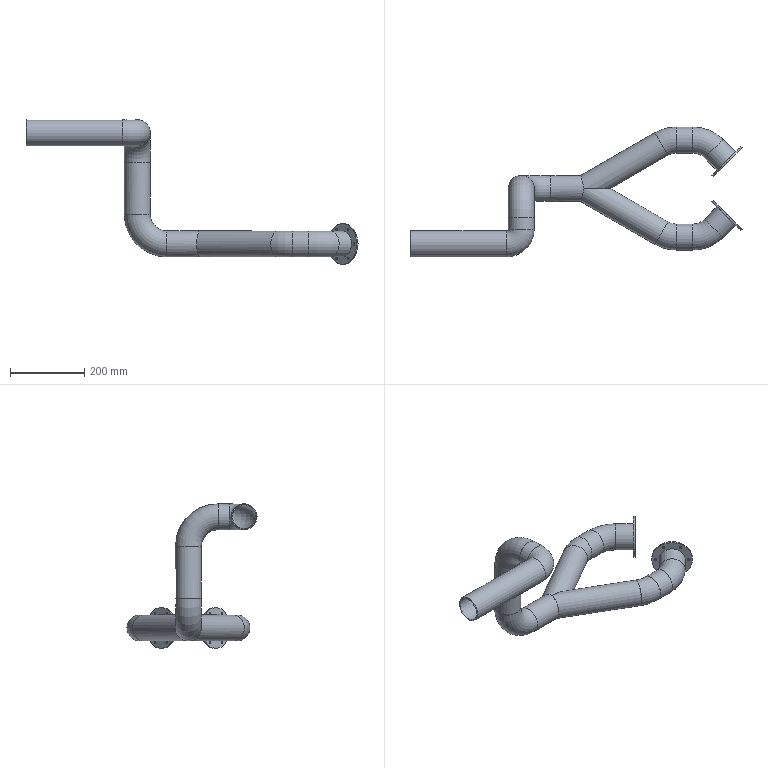Part | STEP file | Pipe Blower | 1 solid | 54 faces | box 895.643 x 351.015 x 390.2 mm | volume 1112047 mm3 | cylinder 34 | torus 14 | plane 5 | cone 1 | commonest cylinder face diameters 6.647 x12 64.2 x10 70.2 x10 110.2 x2